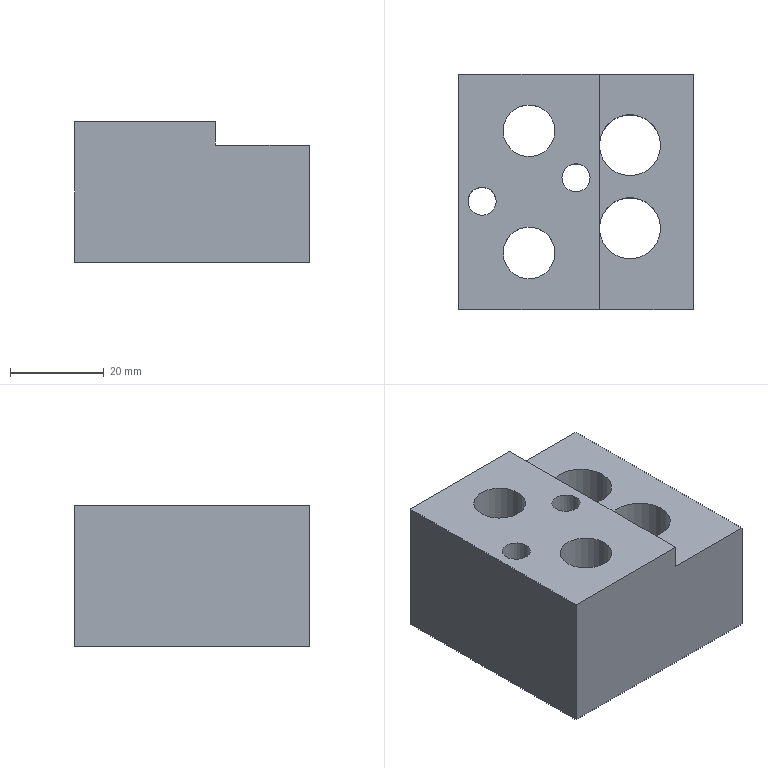Part | NX | features solid 2 | 1 solid | 20 faces | box 50 x 50 x 30 mm | volume 52473 mm3 | plane 12 | cylinder 8 | commonest cylinder face diameters 6 x2 11 x2 13 x2 17.5 x2
STEP:
#1=CARTESIAN_POINT('',(-674.255,-597.733,64.));
#2=VERTEX_POINT('',#1);
#3=CARTESIAN_POINT('',(-680.755,-597.733,64.));
#4=DIRECTION('',(0.,0.,1.));
#5=DIRECTION('',(1.,0.,0.));
#6=AXIS2_PLACEMENT_3D('',#3,#4,#5);
#7=CIRCLE('',#6,6.5);
#8=EDGE_CURVE('',#2,#2,#7,.T.);
#9=ORIENTED_EDGE('',*,*,#8,.T.);
#10=EDGE_LOOP('',(#9));
#11=FACE_BOUND('',#10,.T.);
#12=CARTESIAN_POINT('',(-709.255,-592.,64.));
#13=VERTEX_POINT('',#12);
#14=CARTESIAN_POINT('',(-712.255,-592.,64.));
#15=DIRECTION('',(0.,0.,1.));
#16=DIRECTION('',(1.,0.,0.));
#17=AXIS2_PLACEMENT_3D('',#14,#15,#16);
#18=CIRCLE('',#17,3.);
#19=EDGE_CURVE('',#13,#13,#18,.T.);
#20=ORIENTED_EDGE('',*,*,#19,.T.);
#21=EDGE_LOOP('',(#20));
#22=FACE_BOUND('',#21,.T.);
#23=CARTESIAN_POINT('',(-689.255,-587.,64.));
#24=VERTEX_POINT('',#23);
#25=CARTESIAN_POINT('',(-692.255,-587.,64.));
#26=DIRECTION('',(0.,0.,1.));
#27=DIRECTION('',(1.,0.,0.));
#28=AXIS2_PLACEMENT_3D('',#25,#26,#27);
#29=CIRCLE('',#28,3.);
#30=EDGE_CURVE('',#24,#24,#29,.T.);
#31=ORIENTED_EDGE('',*,*,#30,.T.);
#32=EDGE_LOOP('',(#31));
#33=FACE_BOUND('',#32,.T.);
#34=CARTESIAN_POINT('',(-693.505,-577.,64.));
#35=VERTEX_POINT('',#34);
#36=CARTESIAN_POINT('',(-702.255,-577.,64.));
#37=DIRECTION('',(0.,0.,1.));
#38=DIRECTION('',(1.,0.,0.));
#39=AXIS2_PLACEMENT_3D('',#36,#37,#38);
#40=CIRCLE('',#39,8.75);
#41=EDGE_CURVE('',#35,#35,#40,.T.);
#42=ORIENTED_EDGE('',*,*,#41,.T.);
#43=EDGE_LOOP('',(#42));
#44=FACE_BOUND('',#43,.T.);
#45=CARTESIAN_POINT('',(-693.505,-603.,64.));
#46=VERTEX_POINT('',#45);
#47=CARTESIAN_POINT('',(-702.255,-603.,64.));
#48=DIRECTION('',(0.,0.,1.));
#49=DIRECTION('',(1.,0.,0.));
#50=AXIS2_PLACEMENT_3D('',#47,#48,#49);
#51=CIRCLE('',#50,8.75);
#52=EDGE_CURVE('',#46,#46,#51,.T.);
#53=ORIENTED_EDGE('',*,*,#52,.T.);
#54=EDGE_LOOP('',(#53));
#55=FACE_BOUND('',#54,.T.);
#56=CARTESIAN_POINT('',(-667.255,-565.,64.));
#57=VERTEX_POINT('',#56);
#58=CARTESIAN_POINT('',(-717.255,-565.,64.));
#59=VERTEX_POINT('',#58);
#60=CARTESIAN_POINT('',(-687.255,-565.,64.));
#61=DIRECTION('',(1.,0.,0.));
#62=VECTOR('',#61,1000.);
#63=LINE('',#60,#62);
#64=EDGE_CURVE('',#57,#59,#63,.F.);
#65=ORIENTED_EDGE('',*,*,#64,.F.);
#66=CARTESIAN_POINT('',(-667.255,-615.,64.));
#67=VERTEX_POINT('',#66);
#68=CARTESIAN_POINT('',(-667.255,-584.713,64.));
#69=DIRECTION('',(0.,-1.,0.));
#70=VECTOR('',#69,1000.);
#71=LINE('',#68,#70);
#72=EDGE_CURVE('',#67,#57,#71,.F.);
#73=ORIENTED_EDGE('',*,*,#72,.F.);
#74=CARTESIAN_POINT('',(-717.255,-615.,64.));
#75=VERTEX_POINT('',#74);
#76=CARTESIAN_POINT('',(-687.255,-615.,64.));
#77=DIRECTION('',(1.,0.,0.));
#78=VECTOR('',#77,1000.);
#79=LINE('',#76,#78);
#80=EDGE_CURVE('',#67,#75,#79,.F.);
#81=ORIENTED_EDGE('',*,*,#80,.T.);
#82=CARTESIAN_POINT('',(-717.255,-584.713,64.));
#83=DIRECTION('',(0.,-1.,0.));
#84=VECTOR('',#83,1000.);
#85=LINE('',#82,#84);
#86=EDGE_CURVE('',#75,#59,#85,.F.);
#87=ORIENTED_EDGE('',*,*,#86,.T.);
#88=EDGE_LOOP('',(#65,#73,#81,#87));
#89=FACE_BOUND('',#88,.T.);
#90=CARTESIAN_POINT('',(-674.255,-580.049,64.));
#91=VERTEX_POINT('',#90);
#92=CARTESIAN_POINT('',(-680.755,-580.049,64.));
#93=DIRECTION('',(0.,0.,1.));
#94=DIRECTION('',(1.,0.,0.));
#95=AXIS2_PLACEMENT_3D('',#92,#93,#94);
#96=CIRCLE('',#95,6.5);
#97=EDGE_CURVE('',#91,#91,#96,.T.);
#98=ORIENTED_EDGE('',*,*,#97,.T.);
#99=EDGE_LOOP('',(#98));
#100=FACE_BOUND('',#99,.T.);
#101=CARTESIAN_POINT('',(-687.255,-584.713,64.));
#102=DIRECTION('',(0.,0.,-1.));
#103=DIRECTION('',(0.,1.,0.));
#104=AXIS2_PLACEMENT_3D('',#101,#102,#103);
#105=PLANE('',#104);
#106=ADVANCED_FACE('',(#11,#22,#33,#44,#55,#89,#100),#105,.T.);
#107=CARTESIAN_POINT('',(-687.255,-602.397,94.));
#108=VERTEX_POINT('',#107);
#109=CARTESIAN_POINT('',(-687.255,-602.397,89.));
#110=VERTEX_POINT('',#109);
#111=CARTESIAN_POINT('',(-687.255,-602.397,89.));
#112=CARTESIAN_POINT('',(-687.255,-602.397,90.667));
#113=CARTESIAN_POINT('',(-687.255,-602.397,92.333));
#114=CARTESIAN_POINT('',(-687.255,-602.397,94.));
#115=B_SPLINE_CURVE_WITH_KNOTS('',3,(#111,#112,#113,#114),.UNSPECIFIED.,.F.,.F.,(4,4),(0.,1.),.UNSPECIFIED.);
#116=EDGE_CURVE('',#108,#110,#115,.F.);
#117=ORIENTED_EDGE('',*,*,#116,.F.);
#118=CARTESIAN_POINT('',(-687.255,-615.,94.));
#119=VERTEX_POINT('',#118);
#120=CARTESIAN_POINT('',(-687.255,-580.049,94.));
#121=DIRECTION('',(0.,1.,0.));
#122=VECTOR('',#121,1000.);
#123=LINE('',#120,#122);
#124=EDGE_CURVE('',#119,#108,#123,.T.);
#125=ORIENTED_EDGE('',*,*,#124,.F.);
#126=CARTESIAN_POINT('',(-687.255,-615.,89.));
#127=VERTEX_POINT('',#126);
#128=CARTESIAN_POINT('',(-687.255,-615.,97.));
#129=DIRECTION('',(0.,0.,1.));
#130=VECTOR('',#129,1000.);
#131=LINE('',#128,#130);
#132=EDGE_CURVE('',#127,#119,#131,.T.);
#133=ORIENTED_EDGE('',*,*,#132,.F.);
#134=CARTESIAN_POINT('',(-687.255,-597.733,89.));
#135=DIRECTION('',(0.,1.,0.));
#136=VECTOR('',#135,1000.);
#137=LINE('',#134,#136);
#138=EDGE_CURVE('',#110,#127,#137,.F.);
#139=ORIENTED_EDGE('',*,*,#138,.F.);
#140=EDGE_LOOP('',(#117,#125,#133,#139));
#141=FACE_BOUND('',#140,.T.);
#142=CARTESIAN_POINT('',(-687.255,-575.385,97.));
#143=DIRECTION('',(1.,0.,0.));
#144=DIRECTION('',(0.,0.,-1.));
#145=AXIS2_PLACEMENT_3D('',#142,#143,#144);
#146=PLANE('',#145);
#147=ADVANCED_FACE('',(#141),#146,.T.);
#148=CARTESIAN_POINT('',(-667.255,-565.,89.));
#149=VERTEX_POINT('',#148);
#150=CARTESIAN_POINT('',(-667.255,-565.,64.));
#151=DIRECTION('',(0.,0.,1.));
#152=VECTOR('',#151,1000.);
#153=LINE('',#150,#152);
#154=EDGE_CURVE('',#57,#149,#153,.T.);
#155=ORIENTED_EDGE('',*,*,#154,.F.);
#156=ORIENTED_EDGE('',*,*,#64,.T.);
#157=CARTESIAN_POINT('',(-717.255,-565.,94.));
#158=VERTEX_POINT('',#157);
#159=CARTESIAN_POINT('',(-717.255,-565.,64.));
#160=DIRECTION('',(0.,0.,1.));
#161=VECTOR('',#160,1000.);
#162=LINE('',#159,#161);
#163=EDGE_CURVE('',#59,#158,#162,.T.);
#164=ORIENTED_EDGE('',*,*,#163,.T.);
#165=CARTESIAN_POINT('',(-687.255,-565.,94.));
#166=VERTEX_POINT('',#165);
#167=CARTESIAN_POINT('',(-687.255,-565.,94.));
#168=DIRECTION('',(-1.,0.,0.));
#169=VECTOR('',#168,1000.);
#170=LINE('',#167,#169);
#171=EDGE_CURVE('',#166,#158,#170,.T.);
#172=ORIENTED_EDGE('',*,*,#171,.F.);
#173=CARTESIAN_POINT('',(-687.255,-565.,89.));
#174=VERTEX_POINT('',#173);
#175=CARTESIAN_POINT('',(-687.255,-565.,97.));
#176=DIRECTION('',(0.,0.,1.));
#177=VECTOR('',#176,1000.);
#178=LINE('',#175,#177);
#179=EDGE_CURVE('',#174,#166,#178,.T.);
#180=ORIENTED_EDGE('',*,*,#179,.F.);
#181=CARTESIAN_POINT('',(-680.755,-565.,89.));
#182=DIRECTION('',(-1.,0.,0.));
#183=VECTOR('',#182,1000.);
#184=LINE('',#181,#183);
#185=EDGE_CURVE('',#174,#149,#184,.F.);
#186=ORIENTED_EDGE('',*,*,#185,.T.);
#187=EDGE_LOOP('',(#155,#156,#164,#172,#180,#186));
#188=FACE_BOUND('',#187,.T.);
#189=CARTESIAN_POINT('',(0.,-565.,-0.3931));
#190=DIRECTION('',(0.,1.,0.));
#191=DIRECTION('',(0.,0.,1.));
#192=AXIS2_PLACEMENT_3D('',#189,#190,#191);
#193=PLANE('',#192);
#194=ADVANCED_FACE('',(#188),#193,.T.);
#195=CARTESIAN_POINT('',(-667.255,-615.,89.));
#196=VERTEX_POINT('',#195);
#197=CARTESIAN_POINT('',(-667.255,-615.,64.));
#198=DIRECTION('',(0.,0.,1.));
#199=VECTOR('',#198,1000.);
#200=LINE('',#197,#199);
#201=EDGE_CURVE('',#67,#196,#200,.T.);
#202=ORIENTED_EDGE('',*,*,#201,.T.);
#203=CARTESIAN_POINT('',(-680.755,-615.,89.));
#204=DIRECTION('',(-1.,0.,0.));
#205=VECTOR('',#204,1000.);
#206=LINE('',#203,#205);
#207=EDGE_CURVE('',#127,#196,#206,.F.);
#208=ORIENTED_EDGE('',*,*,#207,.F.);
#209=ORIENTED_EDGE('',*,*,#132,.T.);
#210=CARTESIAN_POINT('',(-717.255,-615.,94.));
#211=VERTEX_POINT('',#210);
#212=CARTESIAN_POINT('',(-687.255,-615.,94.));
#213=DIRECTION('',(-1.,0.,0.));
#214=VECTOR('',#213,1000.);
#215=LINE('',#212,#214);
#216=EDGE_CURVE('',#119,#211,#215,.T.);
#217=ORIENTED_EDGE('',*,*,#216,.T.);
#218=CARTESIAN_POINT('',(-717.255,-615.,64.));
#219=DIRECTION('',(0.,0.,1.));
#220=VECTOR('',#219,1000.);
#221=LINE('',#218,#220);
#222=EDGE_CURVE('',#75,#211,#221,.T.);
#223=ORIENTED_EDGE('',*,*,#222,.F.);
#224=ORIENTED_EDGE('',*,*,#80,.F.);
#225=EDGE_LOOP('',(#202,#208,#209,#217,#223,#224));
#226=FACE_BOUND('',#225,.T.);
#227=CARTESIAN_POINT('',(0.,-615.,-0.3931));
#228=DIRECTION('',(0.,1.,0.));
#229=DIRECTION('',(0.,0.,1.));
#230=AXIS2_PLACEMENT_3D('',#227,#228,#229);
#231=PLANE('',#230);
#232=ADVANCED_FACE('',(#226),#231,.F.);
#233=ORIENTED_EDGE('',*,*,#72,.T.);
#234=ORIENTED_EDGE('',*,*,#154,.T.);
#235=CARTESIAN_POINT('',(-667.255,-584.713,89.));
#236=DIRECTION('',(0.,-1.,0.));
#237=VECTOR('',#236,1000.);
#238=LINE('',#235,#237);
#239=EDGE_CURVE('',#196,#149,#238,.F.);
#240=ORIENTED_EDGE('',*,*,#239,.F.);
#241=ORIENTED_EDGE('',*,*,#201,.F.);
#242=EDGE_LOOP('',(#233,#234,#240,#241));
#243=FACE_BOUND('',#242,.T.);
#244=CARTESIAN_POINT('',(-667.255,-584.713,64.));
#245=DIRECTION('',(1.,0.,0.));
#246=DIRECTION('',(0.,0.,-1.));
#247=AXIS2_PLACEMENT_3D('',#244,#245,#246);
#248=PLANE('',#247);
#249=ADVANCED_FACE('',(#243),#248,.T.);
#250=CARTESIAN_POINT('',(-687.255,-593.069,94.));
#251=VERTEX_POINT('',#250);
#252=CARTESIAN_POINT('',(-687.255,-580.049,94.));
#253=DIRECTION('',(0.,1.,0.));
#254=VECTOR('',#253,1000.);
#255=LINE('',#252,#254);
#256=EDGE_CURVE('',#251,#166,#255,.T.);
#257=ORIENTED_EDGE('',*,*,#256,.T.);
#258=ORIENTED_EDGE('',*,*,#171,.T.);
#259=CARTESIAN_POINT('',(-717.255,-580.049,94.));
#260=DIRECTION('',(0.,1.,0.));
#261=VECTOR('',#260,1000.);
#262=LINE('',#259,#261);
#263=EDGE_CURVE('',#211,#158,#262,.T.);
#264=ORIENTED_EDGE('',*,*,#263,.F.);
#265=ORIENTED_EDGE('',*,*,#216,.F.);
#266=ORIENTED_EDGE('',*,*,#124,.T.);
#267=CARTESIAN_POINT('',(-687.255,-593.069,94.));
#268=DIRECTION('',(0.,1.,0.));
#269=VECTOR('',#268,1000.);
#270=LINE('',#267,#269);
#271=EDGE_CURVE('',#108,#251,#270,.T.);
#272=ORIENTED_EDGE('',*,*,#271,.T.);
#273=EDGE_LOOP('',(#257,#258,#264,#265,#266,#272));
#274=FACE_BOUND('',#273,.T.);
#275=CARTESIAN_POINT('',(-709.255,-592.,94.));
#276=VERTEX_POINT('',#275);
#277=CARTESIAN_POINT('',(-712.255,-592.,94.));
#278=DIRECTION('',(0.,0.,1.));
#279=DIRECTION('',(1.,0.,0.));
#280=AXIS2_PLACEMENT_3D('',#277,#278,#279);
#281=CIRCLE('',#280,3.);
#282=EDGE_CURVE('',#276,#276,#281,.T.);
#283=ORIENTED_EDGE('',*,*,#282,.F.);
#284=EDGE_LOOP('',(#283));
#285=FACE_BOUND('',#284,.T.);
#286=CARTESIAN_POINT('',(-689.255,-587.,94.));
#287=VERTEX_POINT('',#286);
#288=CARTESIAN_POINT('',(-692.255,-587.,94.));
#289=DIRECTION('',(0.,0.,1.));
#290=DIRECTION('',(1.,0.,0.));
#291=AXIS2_PLACEMENT_3D('',#288,#289,#290);
#292=CIRCLE('',#291,3.);
#293=EDGE_CURVE('',#287,#287,#292,.T.);
#294=ORIENTED_EDGE('',*,*,#293,.F.);
#295=EDGE_LOOP('',(#294));
#296=FACE_BOUND('',#295,.T.);
#297=CARTESIAN_POINT('',(-696.755,-577.,94.));
#298=VERTEX_POINT('',#297);
#299=CARTESIAN_POINT('',(-702.255,-577.,94.));
#300=DIRECTION('',(0.,0.,1.));
#301=DIRECTION('',(1.,0.,0.));
#302=AXIS2_PLACEMENT_3D('',#299,#300,#301);
#303=CIRCLE('',#302,5.5);
#304=EDGE_CURVE('',#298,#298,#303,.T.);
#305=ORIENTED_EDGE('',*,*,#304,.F.);
#306=EDGE_LOOP('',(#305));
#307=FACE_BOUND('',#306,.T.);
#308=CARTESIAN_POINT('',(-696.755,-603.,94.));
#309=VERTEX_POINT('',#308);
#310=CARTESIAN_POINT('',(-702.255,-603.,94.));
#311=DIRECTION('',(0.,0.,1.));
#312=DIRECTION('',(1.,0.,0.));
#313=AXIS2_PLACEMENT_3D('',#310,#311,#312);
#314=CIRCLE('',#313,5.5);
#315=EDGE_CURVE('',#309,#309,#314,.T.);
#316=ORIENTED_EDGE('',*,*,#315,.F.);
#317=EDGE_LOOP('',(#316));
#318=FACE_BOUND('',#317,.T.);
#319=CARTESIAN_POINT('',(-687.255,-580.049,94.));
#320=DIRECTION('',(0.,0.,1.));
#321=DIRECTION('',(1.,0.,0.));
#322=AXIS2_PLACEMENT_3D('',#319,#320,#321);
#323=PLANE('',#322);
#324=ADVANCED_FACE('',(#274,#285,#296,#307,#318),#323,.T.);
#325=CARTESIAN_POINT('',(-687.255,-580.049,89.));
#326=VERTEX_POINT('',#325);
#327=CARTESIAN_POINT('',(-687.255,-597.733,89.));
#328=DIRECTION('',(0.,1.,0.));
#329=VECTOR('',#328,1000.);
#330=LINE('',#327,#329);
#331=EDGE_CURVE('',#174,#326,#330,.F.);
#332=ORIENTED_EDGE('',*,*,#331,.F.);
#333=ORIENTED_EDGE('',*,*,#179,.T.);
#334=ORIENTED_EDGE('',*,*,#256,.F.);
#335=CARTESIAN_POINT('',(-687.255,-593.069,89.));
#336=VERTEX_POINT('',#335);
#337=CARTESIAN_POINT('',(-687.255,-593.069,94.));
#338=CARTESIAN_POINT('',(-687.255,-593.069,92.333));
#339=CARTESIAN_POINT('',(-687.255,-593.069,90.667));
#340=CARTESIAN_POINT('',(-687.255,-593.069,89.));
#341=B_SPLINE_CURVE_WITH_KNOTS('',3,(#337,#338,#339,#340),.UNSPECIFIED.,.F.,.F.,(4,4),(0.,1.),.UNSPECIFIED.);
#342=EDGE_CURVE('',#251,#336,#341,.T.);
#343=ORIENTED_EDGE('',*,*,#342,.T.);
#344=CARTESIAN_POINT('',(-687.255,-597.733,89.));
#345=DIRECTION('',(0.,1.,0.));
#346=VECTOR('',#345,1000.);
#347=LINE('',#344,#346);
#348=EDGE_CURVE('',#326,#336,#347,.F.);
#349=ORIENTED_EDGE('',*,*,#348,.F.);
#350=EDGE_LOOP('',(#332,#333,#334,#343,#349));
#351=FACE_BOUND('',#350,.T.);
#352=CARTESIAN_POINT('',(-687.255,-575.385,97.));
#353=DIRECTION('',(1.,0.,0.));
#354=DIRECTION('',(0.,0.,-1.));
#355=AXIS2_PLACEMENT_3D('',#352,#353,#354);
#356=PLANE('',#355);
#357=ADVANCED_FACE('',(#351),#356,.T.);
#358=ORIENTED_EDGE('',*,*,#163,.F.);
#359=ORIENTED_EDGE('',*,*,#86,.F.);
#360=ORIENTED_EDGE('',*,*,#222,.T.);
#361=ORIENTED_EDGE('',*,*,#263,.T.);
#362=EDGE_LOOP('',(#358,#359,#360,#361));
#363=FACE_BOUND('',#362,.T.);
#364=CARTESIAN_POINT('',(-717.255,-584.713,64.));
#365=DIRECTION('',(1.,0.,0.));
#366=DIRECTION('',(0.,0.,-1.));
#367=AXIS2_PLACEMENT_3D('',#364,#365,#366);
#368=PLANE('',#367);
#369=ADVANCED_FACE('',(#363),#368,.F.);
#370=CARTESIAN_POINT('',(-687.255,-597.733,89.));
#371=VERTEX_POINT('',#370);
#372=CARTESIAN_POINT('',(-687.255,-597.733,89.));
#373=DIRECTION('',(0.,1.,0.));
#374=VECTOR('',#373,1000.);
#375=LINE('',#372,#374);
#376=EDGE_CURVE('',#371,#336,#375,.T.);
#377=ORIENTED_EDGE('',*,*,#376,.F.);
#378=CARTESIAN_POINT('',(-680.755,-597.733,89.));
#379=DIRECTION('',(0.,0.,1.));
#380=DIRECTION('',(1.,0.,0.));
#381=AXIS2_PLACEMENT_3D('',#378,#379,#380);
#382=CIRCLE('',#381,6.5);
#383=EDGE_CURVE('',#371,#371,#382,.T.);
#384=ORIENTED_EDGE('',*,*,#383,.F.);
#385=CARTESIAN_POINT('',(-687.255,-597.733,89.));
#386=DIRECTION('',(0.,1.,0.));
#387=VECTOR('',#386,1000.);
#388=LINE('',#385,#387);
#389=EDGE_CURVE('',#110,#371,#388,.T.);
#390=ORIENTED_EDGE('',*,*,#389,.F.);
#391=ORIENTED_EDGE('',*,*,#138,.T.);
#392=ORIENTED_EDGE('',*,*,#207,.T.);
#393=ORIENTED_EDGE('',*,*,#239,.T.);
#394=ORIENTED_EDGE('',*,*,#185,.F.);
#395=ORIENTED_EDGE('',*,*,#331,.T.);
#396=CARTESIAN_POINT('',(-680.755,-580.049,89.));
#397=DIRECTION('',(0.,0.,-1.));
#398=DIRECTION('',(-1.,0.,0.));
#399=AXIS2_PLACEMENT_3D('',#396,#397,#398);
#400=CIRCLE('',#399,6.5);
#401=EDGE_CURVE('',#326,#326,#400,.F.);
#402=ORIENTED_EDGE('',*,*,#401,.F.);
#403=ORIENTED_EDGE('',*,*,#348,.T.);
#404=EDGE_LOOP('',(#377,#384,#390,#391,#392,#393,#394,#395,#402,#403));
#405=FACE_BOUND('',#404,.T.);
#406=CARTESIAN_POINT('',(-680.755,-597.733,89.));
#407=DIRECTION('',(0.,0.,1.));
#408=DIRECTION('',(1.,0.,0.));
#409=AXIS2_PLACEMENT_3D('',#406,#407,#408);
#410=PLANE('',#409);
#411=ADVANCED_FACE('',(#405),#410,.T.);
#412=ORIENTED_EDGE('',*,*,#315,.T.);
#413=EDGE_LOOP('',(#412));
#414=FACE_BOUND('',#413,.T.);
#415=CARTESIAN_POINT('',(-707.755,-603.,76.));
#416=VERTEX_POINT('',#415);
#417=CARTESIAN_POINT('',(-702.255,-603.,76.));
#418=DIRECTION('',(0.,0.,-1.));
#419=DIRECTION('',(-1.,0.,0.));
#420=AXIS2_PLACEMENT_3D('',#417,#418,#419);
#421=CIRCLE('',#420,5.5);
#422=EDGE_CURVE('',#416,#416,#421,.F.);
#423=ORIENTED_EDGE('',*,*,#422,.F.);
#424=EDGE_LOOP('',(#423));
#425=FACE_BOUND('',#424,.T.);
#426=CARTESIAN_POINT('',(-702.255,-603.,114.));
#427=DIRECTION('',(0.,0.,1.));
#428=DIRECTION('',(1.,0.,0.));
#429=AXIS2_PLACEMENT_3D('',#426,#427,#428);
#430=CYLINDRICAL_SURFACE('',#429,5.5);
#431=ADVANCED_FACE('',(#414,#425),#430,.F.);
#432=ORIENTED_EDGE('',*,*,#422,.T.);
#433=EDGE_LOOP('',(#432));
#434=FACE_BOUND('',#433,.T.);
#435=CARTESIAN_POINT('',(-711.005,-603.,76.));
#436=VERTEX_POINT('',#435);
#437=CARTESIAN_POINT('',(-702.255,-603.,76.));
#438=DIRECTION('',(0.,0.,-1.));
#439=DIRECTION('',(-1.,0.,0.));
#440=AXIS2_PLACEMENT_3D('',#437,#438,#439);
#441=CIRCLE('',#440,8.75);
#442=EDGE_CURVE('',#436,#436,#441,.F.);
#443=ORIENTED_EDGE('',*,*,#442,.F.);
#444=EDGE_LOOP('',(#443));
#445=FACE_BOUND('',#444,.T.);
#446=CARTESIAN_POINT('',(-702.255,-603.,76.));
#447=DIRECTION('',(0.,0.,1.));
#448=DIRECTION('',(1.,0.,0.));
#449=AXIS2_PLACEMENT_3D('',#446,#447,#448);
#450=PLANE('',#449);
#451=ADVANCED_FACE('',(#434,#445),#450,.F.);
#452=ORIENTED_EDGE('',*,*,#442,.T.);
#453=EDGE_LOOP('',(#452));
#454=FACE_BOUND('',#453,.T.);
#455=ORIENTED_EDGE('',*,*,#52,.F.);
#456=EDGE_LOOP('',(#455));
#457=FACE_BOUND('',#456,.T.);
#458=CARTESIAN_POINT('',(-702.255,-603.,64.));
#459=DIRECTION('',(0.,0.,1.));
#460=DIRECTION('',(1.,0.,0.));
#461=AXIS2_PLACEMENT_3D('',#458,#459,#460);
#462=CYLINDRICAL_SURFACE('',#461,8.75);
#463=ADVANCED_FACE('',(#454,#457),#462,.F.);
#464=ORIENTED_EDGE('',*,*,#304,.T.);
#465=EDGE_LOOP('',(#464));
#466=FACE_BOUND('',#465,.T.);
#467=CARTESIAN_POINT('',(-707.755,-577.,76.));
#468=VERTEX_POINT('',#467);
#469=CARTESIAN_POINT('',(-702.255,-577.,76.));
#470=DIRECTION('',(0.,0.,-1.));
#471=DIRECTION('',(-1.,0.,0.));
#472=AXIS2_PLACEMENT_3D('',#469,#470,#471);
#473=CIRCLE('',#472,5.5);
#474=EDGE_CURVE('',#468,#468,#473,.F.);
#475=ORIENTED_EDGE('',*,*,#474,.F.);
#476=EDGE_LOOP('',(#475));
#477=FACE_BOUND('',#476,.T.);
#478=CARTESIAN_POINT('',(-702.255,-577.,114.));
#479=DIRECTION('',(0.,0.,1.));
#480=DIRECTION('',(1.,0.,0.));
#481=AXIS2_PLACEMENT_3D('',#478,#479,#480);
#482=CYLINDRICAL_SURFACE('',#481,5.5);
#483=ADVANCED_FACE('',(#466,#477),#482,.F.);
#484=ORIENTED_EDGE('',*,*,#474,.T.);
#485=EDGE_LOOP('',(#484));
#486=FACE_BOUND('',#485,.T.);
#487=CARTESIAN_POINT('',(-711.005,-577.,76.));
#488=VERTEX_POINT('',#487);
#489=CARTESIAN_POINT('',(-702.255,-577.,76.));
#490=DIRECTION('',(0.,0.,-1.));
#491=DIRECTION('',(-1.,0.,0.));
#492=AXIS2_PLACEMENT_3D('',#489,#490,#491);
#493=CIRCLE('',#492,8.75);
#494=EDGE_CURVE('',#488,#488,#493,.F.);
#495=ORIENTED_EDGE('',*,*,#494,.F.);
#496=EDGE_LOOP('',(#495));
#497=FACE_BOUND('',#496,.T.);
#498=CARTESIAN_POINT('',(-702.255,-577.,76.));
#499=DIRECTION('',(0.,0.,1.));
#500=DIRECTION('',(1.,0.,0.));
#501=AXIS2_PLACEMENT_3D('',#498,#499,#500);
#502=PLANE('',#501);
#503=ADVANCED_FACE('',(#486,#497),#502,.F.);
#504=ORIENTED_EDGE('',*,*,#494,.T.);
#505=EDGE_LOOP('',(#504));
#506=FACE_BOUND('',#505,.T.);
#507=ORIENTED_EDGE('',*,*,#41,.F.);
#508=EDGE_LOOP('',(#507));
#509=FACE_BOUND('',#508,.T.);
#510=CARTESIAN_POINT('',(-702.255,-577.,64.));
#511=DIRECTION('',(0.,0.,1.));
#512=DIRECTION('',(1.,0.,0.));
#513=AXIS2_PLACEMENT_3D('',#510,#511,#512);
#514=CYLINDRICAL_SURFACE('',#513,8.75);
#515=ADVANCED_FACE('',(#506,#509),#514,.F.);
#516=ORIENTED_EDGE('',*,*,#293,.T.);
#517=EDGE_LOOP('',(#516));
#518=FACE_BOUND('',#517,.T.);
#519=ORIENTED_EDGE('',*,*,#30,.F.);
#520=EDGE_LOOP('',(#519));
#521=FACE_BOUND('',#520,.T.);
#522=CARTESIAN_POINT('',(-692.255,-587.,64.));
#523=DIRECTION('',(0.,0.,1.));
#524=DIRECTION('',(1.,0.,0.));
#525=AXIS2_PLACEMENT_3D('',#522,#523,#524);
#526=CYLINDRICAL_SURFACE('',#525,3.);
#527=ADVANCED_FACE('',(#518,#521),#526,.F.);
#528=ORIENTED_EDGE('',*,*,#282,.T.);
#529=EDGE_LOOP('',(#528));
#530=FACE_BOUND('',#529,.T.);
#531=ORIENTED_EDGE('',*,*,#19,.F.);
#532=EDGE_LOOP('',(#531));
#533=FACE_BOUND('',#532,.T.);
#534=CARTESIAN_POINT('',(-712.255,-592.,64.));
#535=DIRECTION('',(0.,0.,1.));
#536=DIRECTION('',(1.,0.,0.));
#537=AXIS2_PLACEMENT_3D('',#534,#535,#536);
#538=CYLINDRICAL_SURFACE('',#537,3.);
#539=ADVANCED_FACE('',(#530,#533),#538,.F.);
#540=ORIENTED_EDGE('',*,*,#383,.T.);
#541=EDGE_LOOP('',(#540));
#542=FACE_BOUND('',#541,.T.);
#543=ORIENTED_EDGE('',*,*,#8,.F.);
#544=EDGE_LOOP('',(#543));
#545=FACE_BOUND('',#544,.T.);
#546=CARTESIAN_POINT('',(-680.755,-597.733,94.));
#547=DIRECTION('',(0.,0.,-1.));
#548=DIRECTION('',(-1.,0.,0.));
#549=AXIS2_PLACEMENT_3D('',#546,#547,#548);
#550=CYLINDRICAL_SURFACE('',#549,6.5);
#551=ADVANCED_FACE('',(#542,#545),#550,.F.);
#552=ORIENTED_EDGE('',*,*,#116,.T.);
#553=ORIENTED_EDGE('',*,*,#389,.T.);
#554=ORIENTED_EDGE('',*,*,#376,.T.);
#555=ORIENTED_EDGE('',*,*,#342,.F.);
#556=ORIENTED_EDGE('',*,*,#271,.F.);
#557=EDGE_LOOP('',(#552,#553,#554,#555,#556));
#558=FACE_BOUND('',#557,.T.);
#559=CARTESIAN_POINT('',(-687.255,-593.069,97.));
#560=DIRECTION('',(1.,0.,0.));
#561=DIRECTION('',(0.,1.,0.));
#562=AXIS2_PLACEMENT_3D('',#559,#560,#561);
#563=PLANE('',#562);
#564=ADVANCED_FACE('',(#558),#563,.T.);
#565=ORIENTED_EDGE('',*,*,#401,.T.);
#566=EDGE_LOOP('',(#565));
#567=FACE_BOUND('',#566,.T.);
#568=ORIENTED_EDGE('',*,*,#97,.F.);
#569=EDGE_LOOP('',(#568));
#570=FACE_BOUND('',#569,.T.);
#571=CARTESIAN_POINT('',(-680.755,-580.049,94.));
#572=DIRECTION('',(0.,0.,-1.));
#573=DIRECTION('',(-1.,0.,0.));
#574=AXIS2_PLACEMENT_3D('',#571,#572,#573);
#575=CYLINDRICAL_SURFACE('',#574,6.5);
#576=ADVANCED_FACE('',(#567,#570),#575,.F.);
#577=CLOSED_SHELL('',(#106,#147,#194,#232,#249,#324,#357,#369,#411,#431,#451,#463,#483,#503,#515,#527,#539,#551,#564,#576));
#578=MANIFOLD_SOLID_BREP('',#577);
#579=(LENGTH_UNIT()NAMED_UNIT(*)SI_UNIT(.MILLI.,.METRE.));
#580=UNCERTAINTY_MEASURE_WITH_UNIT(LENGTH_MEASURE(0.0508),#579,'','');
#581=(NAMED_UNIT(*)PLANE_ANGLE_UNIT()SI_UNIT($,.RADIAN.));
#582=(NAMED_UNIT(*)SI_UNIT($,.STERADIAN.)SOLID_ANGLE_UNIT());
#583=(GEOMETRIC_REPRESENTATION_CONTEXT(3)GLOBAL_UNCERTAINTY_ASSIGNED_CONTEXT((#580))GLOBAL_UNIT_ASSIGNED_CONTEXT((#579,#581,#582))REPRESENTATION_CONTEXT('',''));
#584=ADVANCED_BREP_SHAPE_REPRESENTATION('',(#578),#583);